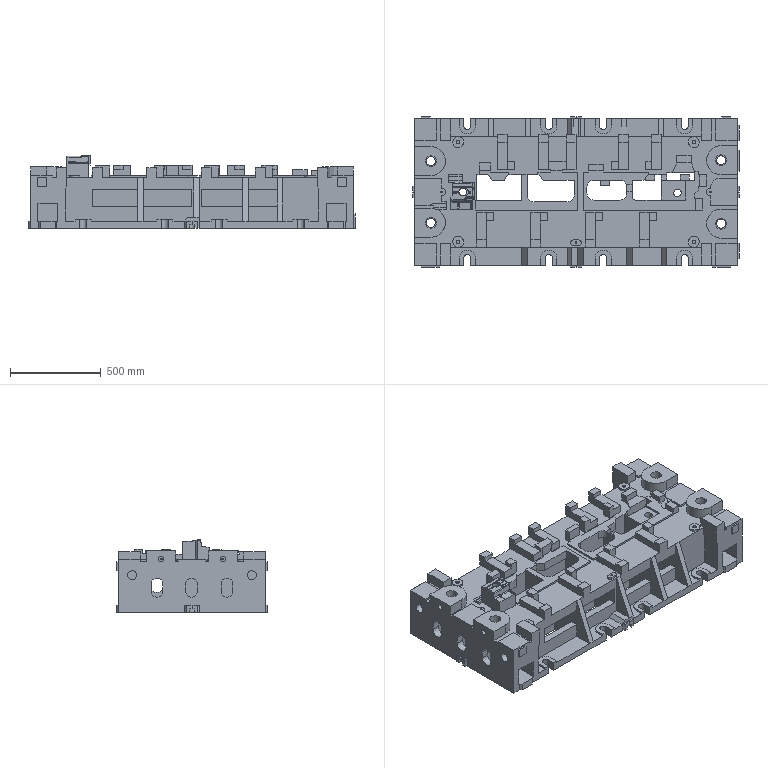Part | NX | features solid 2 | 1 solid | 871 faces | box 1800 x 830 x 402.213 mm | volume 167101651 mm3 | plane 708 | cylinder 121 | spline 39 | cone 3 | commonest cylinder face diameters 60 x30 80 x14 40 x12 10 x11 12 x10 30 x9